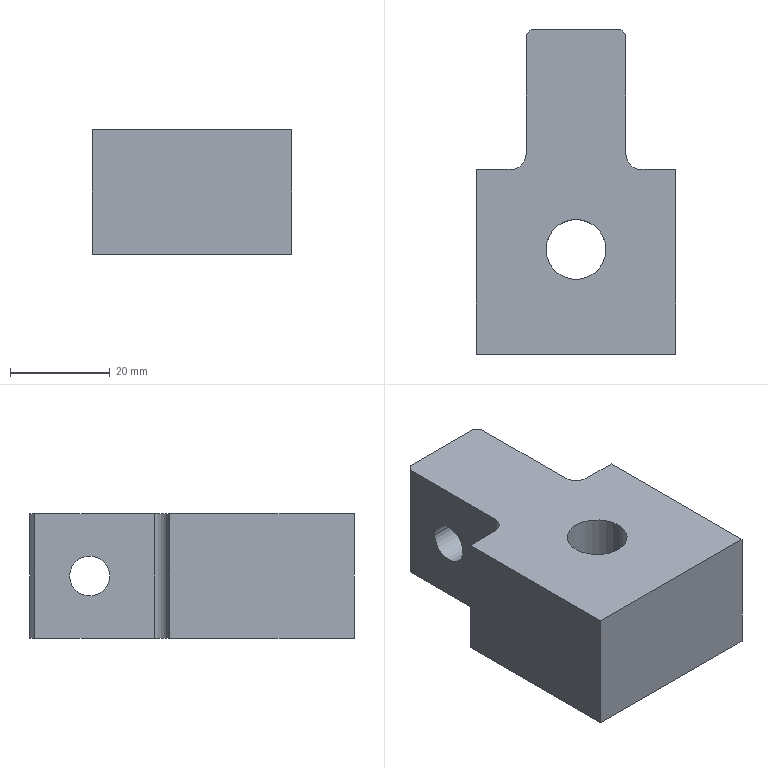Part | STEP file | Chain joint | 1 solid | 18 faces | box 40 x 65 x 25 mm | volume 47239 mm3 | plane 12 | cylinder 6 | commonest cylinder face diameters 6 x2 8 x2 12 x2
STEP:
#1=CARTESIAN_POINT('',(0.,0.,0.));
#2=DIRECTION('',(0.,0.,1.));
#3=DIRECTION('',(1.,0.,0.));
#4=AXIS2_PLACEMENT_3D('',#1,#2,#3);
#5=CARTESIAN_POINT('',(10.,57.,12.5));
#6=VERTEX_POINT('',#5);
#7=CARTESIAN_POINT('',(30.,57.,12.5));
#8=VERTEX_POINT('',#7);
#9=CARTESIAN_POINT('',(0.,57.,12.5));
#10=DIRECTION('',(1.,0.,0.));
#11=VECTOR('',#10,1.);
#12=LINE('',#9,#11);
#13=CARTESIAN_POINT('',(0.,53.,12.5));
#14=DIRECTION('',(1.,0.,0.));
#15=DIRECTION('',(0.,1.,0.));
#16=AXIS2_PLACEMENT_3D('',#13,#14,#15);
#17=CYLINDRICAL_SURFACE('',#16,4.);
#18=CARTESIAN_POINT('',(6.283,0.));
#19=DIRECTION('',(0.,1.));
#20=VECTOR('',#19,1.);
#21=LINE('',#18,#20);
#22=(GEOMETRIC_REPRESENTATION_CONTEXT(2)PARAMETRIC_REPRESENTATION_CONTEXT()REPRESENTATION_CONTEXT('',''));
#23=DEFINITIONAL_REPRESENTATION('',(#21),#22);
#24=PCURVE('',#17,#23);
#25=CARTESIAN_POINT('',(0.,53.,12.5));
#26=DIRECTION('',(1.,0.,0.));
#27=DIRECTION('',(0.,1.,0.));
#28=AXIS2_PLACEMENT_3D('',#25,#26,#27);
#29=CYLINDRICAL_SURFACE('',#28,4.);
#30=CARTESIAN_POINT('',(0.,0.));
#31=DIRECTION('',(0.,1.));
#32=VECTOR('',#31,1.);
#33=LINE('',#30,#32);
#34=(GEOMETRIC_REPRESENTATION_CONTEXT(2)PARAMETRIC_REPRESENTATION_CONTEXT()REPRESENTATION_CONTEXT('',''));
#35=DEFINITIONAL_REPRESENTATION('',(#33),#34);
#36=PCURVE('',#29,#35);
#37=SURFACE_CURVE('',#12,(#24,#36),.PCURVE_S1.);
#38=EDGE_CURVE('',#6,#8,#37,.T.);
#39=ORIENTED_EDGE('',*,*,#38,.T.);
#40=CARTESIAN_POINT('',(30.,49.,12.5));
#41=VERTEX_POINT('',#40);
#42=CARTESIAN_POINT('',(30.,53.,12.5));
#43=DIRECTION('',(1.,0.,0.));
#44=DIRECTION('',(0.,1.,0.));
#45=AXIS2_PLACEMENT_3D('',#42,#43,#44);
#46=CIRCLE('',#45,4.);
#47=CARTESIAN_POINT('',(0.,30.));
#48=DIRECTION('',(1.,0.));
#49=VECTOR('',#48,1.);
#50=LINE('',#47,#49);
#51=(GEOMETRIC_REPRESENTATION_CONTEXT(2)PARAMETRIC_REPRESENTATION_CONTEXT()REPRESENTATION_CONTEXT('',''));
#52=DEFINITIONAL_REPRESENTATION('',(#50),#51);
#53=PCURVE('',#17,#52);
#54=CARTESIAN_POINT('',(30.,65.,25.));
#55=DIRECTION('',(-1.,0.,0.));
#56=DIRECTION('',(0.,-1.,0.));
#57=AXIS2_PLACEMENT_3D('',#54,#55,#56);
#58=PLANE('',#57);
#59=CARTESIAN_POINT('',(8.,-12.5));
#60=CARTESIAN_POINT('',(8.,-5.572));
#61=CARTESIAN_POINT('',(14.,-9.036));
#62=CARTESIAN_POINT('',(20.,-12.5));
#63=CARTESIAN_POINT('',(14.,-15.964));
#64=CARTESIAN_POINT('',(8.,-19.428));
#65=CARTESIAN_POINT('',(8.,-12.5));
#66=(BOUNDED_CURVE()B_SPLINE_CURVE(2,(#59,#60,#61,#62,#63,#64,#65),.UNSPECIFIED.,.T.,.F.)B_SPLINE_CURVE_WITH_KNOTS((1,2,2,2,2,1),(-2.094,0.,2.094,4.189,6.283,8.378),.UNSPECIFIED.)CURVE()GEOMETRIC_REPRESENTATION_ITEM()RATIONAL_B_SPLINE_CURVE((1.,0.5,1.,0.5,1.,0.5,1.))REPRESENTATION_ITEM(''));
#67=(GEOMETRIC_REPRESENTATION_CONTEXT(2)PARAMETRIC_REPRESENTATION_CONTEXT()REPRESENTATION_CONTEXT('',''));
#68=DEFINITIONAL_REPRESENTATION('',(#66),#67);
#69=PCURVE('',#58,#68);
#70=SURFACE_CURVE('',#46,(#53,#69),.PCURVE_S1.);
#71=EDGE_CURVE('',#41,#8,#70,.T.);
#72=ORIENTED_EDGE('',*,*,#71,.F.);
#73=CARTESIAN_POINT('',(10.,49.,12.5));
#74=VERTEX_POINT('',#73);
#75=CARTESIAN_POINT('',(0.,49.,12.5));
#76=DIRECTION('',(1.,0.,0.));
#77=VECTOR('',#76,1.);
#78=LINE('',#75,#77);
#79=CARTESIAN_POINT('',(3.142,0.));
#80=DIRECTION('',(0.,1.));
#81=VECTOR('',#80,1.);
#82=LINE('',#79,#81);
#83=(GEOMETRIC_REPRESENTATION_CONTEXT(2)PARAMETRIC_REPRESENTATION_CONTEXT()REPRESENTATION_CONTEXT('',''));
#84=DEFINITIONAL_REPRESENTATION('',(#82),#83);
#85=PCURVE('',#17,#84);
#86=CARTESIAN_POINT('',(3.142,0.));
#87=DIRECTION('',(0.,1.));
#88=VECTOR('',#87,1.);
#89=LINE('',#86,#88);
#90=(GEOMETRIC_REPRESENTATION_CONTEXT(2)PARAMETRIC_REPRESENTATION_CONTEXT()REPRESENTATION_CONTEXT('',''));
#91=DEFINITIONAL_REPRESENTATION('',(#89),#90);
#92=PCURVE('',#29,#91);
#93=SURFACE_CURVE('',#78,(#85,#92),.PCURVE_S1.);
#94=EDGE_CURVE('',#74,#41,#93,.T.);
#95=ORIENTED_EDGE('',*,*,#94,.F.);
#96=CARTESIAN_POINT('',(10.,53.,12.5));
#97=DIRECTION('',(1.,0.,0.));
#98=DIRECTION('',(0.,0.,-1.));
#99=AXIS2_PLACEMENT_3D('',#96,#97,#98);
#100=CIRCLE('',#99,4.);
#101=CARTESIAN_POINT('',(-1.571,10.));
#102=DIRECTION('',(1.,0.));
#103=VECTOR('',#102,1.);
#104=LINE('',#101,#103);
#105=(GEOMETRIC_REPRESENTATION_CONTEXT(2)PARAMETRIC_REPRESENTATION_CONTEXT()REPRESENTATION_CONTEXT('',''));
#106=DEFINITIONAL_REPRESENTATION('',(#104),#105);
#107=PCURVE('',#17,#106);
#108=CARTESIAN_POINT('',(10.,37.,25.));
#109=DIRECTION('',(1.,0.,0.));
#110=DIRECTION('',(0.,0.,-1.));
#111=AXIS2_PLACEMENT_3D('',#108,#109,#110);
#112=PLANE('',#111);
#113=CARTESIAN_POINT('',(12.5,16.));
#114=DIRECTION('',(1.,0.));
#115=AXIS2_PLACEMENT_2D('',#113,#114);
#116=CIRCLE('',#115,4.);
#117=(GEOMETRIC_REPRESENTATION_CONTEXT(2)PARAMETRIC_REPRESENTATION_CONTEXT()REPRESENTATION_CONTEXT('',''));
#118=DEFINITIONAL_REPRESENTATION('',(#116),#117);
#119=PCURVE('',#112,#118);
#120=SURFACE_CURVE('',#100,(#107,#119),.PCURVE_S1.);
#121=EDGE_CURVE('',#74,#6,#120,.T.);
#122=ORIENTED_EDGE('',*,*,#121,.T.);
#123=EDGE_LOOP('',(#39,#72,#95,#122));
#124=FACE_BOUND('',#123,.F.);
#125=ADVANCED_FACE('',(#124),#17,.F.);
#126=CARTESIAN_POINT('',(14.,21.,25.));
#127=VERTEX_POINT('',#126);
#128=CARTESIAN_POINT('',(14.,21.,0.));
#129=VERTEX_POINT('',#128);
#130=CARTESIAN_POINT('',(14.,21.,25.));
#131=DIRECTION('',(0.,0.,-1.));
#132=VECTOR('',#131,1.);
#133=LINE('',#130,#132);
#134=CARTESIAN_POINT('',(20.,21.,25.));
#135=DIRECTION('',(0.,0.,-1.));
#136=DIRECTION('',(-1.,0.,0.));
#137=AXIS2_PLACEMENT_3D('',#134,#135,#136);
#138=CYLINDRICAL_SURFACE('',#137,6.);
#139=CARTESIAN_POINT('',(6.283,0.));
#140=DIRECTION('',(0.,1.));
#141=VECTOR('',#140,1.);
#142=LINE('',#139,#141);
#143=(GEOMETRIC_REPRESENTATION_CONTEXT(2)PARAMETRIC_REPRESENTATION_CONTEXT()REPRESENTATION_CONTEXT('',''));
#144=DEFINITIONAL_REPRESENTATION('',(#142),#143);
#145=PCURVE('',#138,#144);
#146=CARTESIAN_POINT('',(20.,21.,25.));
#147=DIRECTION('',(0.,0.,-1.));
#148=DIRECTION('',(-1.,0.,0.));
#149=AXIS2_PLACEMENT_3D('',#146,#147,#148);
#150=CYLINDRICAL_SURFACE('',#149,6.);
#151=CARTESIAN_POINT('',(0.,0.));
#152=DIRECTION('',(0.,1.));
#153=VECTOR('',#152,1.);
#154=LINE('',#151,#153);
#155=(GEOMETRIC_REPRESENTATION_CONTEXT(2)PARAMETRIC_REPRESENTATION_CONTEXT()REPRESENTATION_CONTEXT('',''));
#156=DEFINITIONAL_REPRESENTATION('',(#154),#155);
#157=PCURVE('',#150,#156);
#158=SURFACE_CURVE('',#133,(#145,#157),.PCURVE_S1.);
#159=EDGE_CURVE('',#127,#129,#158,.T.);
#160=ORIENTED_EDGE('',*,*,#159,.T.);
#161=CARTESIAN_POINT('',(26.,21.,0.));
#162=VERTEX_POINT('',#161);
#163=CARTESIAN_POINT('',(20.,21.,0.));
#164=DIRECTION('',(0.,0.,1.));
#165=DIRECTION('',(1.,0.,0.));
#166=AXIS2_PLACEMENT_3D('',#163,#164,#165);
#167=CIRCLE('',#166,6.);
#168=CARTESIAN_POINT('',(9.425,25.));
#169=DIRECTION('',(-1.,0.));
#170=VECTOR('',#169,1.);
#171=LINE('',#168,#170);
#172=(GEOMETRIC_REPRESENTATION_CONTEXT(2)PARAMETRIC_REPRESENTATION_CONTEXT()REPRESENTATION_CONTEXT('',''));
#173=DEFINITIONAL_REPRESENTATION('',(#171),#172);
#174=PCURVE('',#138,#173);
#175=CARTESIAN_POINT('',(0.,0.,0.));
#176=DIRECTION('',(0.,0.,-1.));
#177=DIRECTION('',(-1.,0.,0.));
#178=AXIS2_PLACEMENT_3D('',#175,#176,#177);
#179=PLANE('',#178);
#180=CARTESIAN_POINT('',(-26.,21.));
#181=CARTESIAN_POINT('',(-26.,31.392));
#182=CARTESIAN_POINT('',(-17.,26.196));
#183=CARTESIAN_POINT('',(-8.,21.));
#184=CARTESIAN_POINT('',(-17.,15.804));
#185=CARTESIAN_POINT('',(-26.,10.608));
#186=CARTESIAN_POINT('',(-26.,21.));
#187=(BOUNDED_CURVE()B_SPLINE_CURVE(2,(#180,#181,#182,#183,#184,#185,#186),.UNSPECIFIED.,.T.,.F.)B_SPLINE_CURVE_WITH_KNOTS((1,2,2,2,2,1),(-2.094,0.,2.094,4.189,6.283,8.378),.UNSPECIFIED.)CURVE()GEOMETRIC_REPRESENTATION_ITEM()RATIONAL_B_SPLINE_CURVE((1.,0.5,1.,0.5,1.,0.5,1.))REPRESENTATION_ITEM(''));
#188=(GEOMETRIC_REPRESENTATION_CONTEXT(2)PARAMETRIC_REPRESENTATION_CONTEXT()REPRESENTATION_CONTEXT('',''));
#189=DEFINITIONAL_REPRESENTATION('',(#187),#188);
#190=PCURVE('',#179,#189);
#191=SURFACE_CURVE('',#167,(#174,#190),.PCURVE_S1.);
#192=EDGE_CURVE('',#129,#162,#191,.T.);
#193=ORIENTED_EDGE('',*,*,#192,.T.);
#194=CARTESIAN_POINT('',(26.,21.,25.));
#195=VERTEX_POINT('',#194);
#196=CARTESIAN_POINT('',(26.,21.,25.));
#197=DIRECTION('',(0.,0.,-1.));
#198=VECTOR('',#197,1.);
#199=LINE('',#196,#198);
#200=CARTESIAN_POINT('',(3.142,0.));
#201=DIRECTION('',(0.,1.));
#202=VECTOR('',#201,1.);
#203=LINE('',#200,#202);
#204=(GEOMETRIC_REPRESENTATION_CONTEXT(2)PARAMETRIC_REPRESENTATION_CONTEXT()REPRESENTATION_CONTEXT('',''));
#205=DEFINITIONAL_REPRESENTATION('',(#203),#204);
#206=PCURVE('',#138,#205);
#207=CARTESIAN_POINT('',(3.142,0.));
#208=DIRECTION('',(0.,1.));
#209=VECTOR('',#208,1.);
#210=LINE('',#207,#209);
#211=(GEOMETRIC_REPRESENTATION_CONTEXT(2)PARAMETRIC_REPRESENTATION_CONTEXT()REPRESENTATION_CONTEXT('',''));
#212=DEFINITIONAL_REPRESENTATION('',(#210),#211);
#213=PCURVE('',#150,#212);
#214=SURFACE_CURVE('',#199,(#206,#213),.PCURVE_S1.);
#215=EDGE_CURVE('',#195,#162,#214,.T.);
#216=ORIENTED_EDGE('',*,*,#215,.F.);
#217=CARTESIAN_POINT('',(20.,21.,25.));
#218=DIRECTION('',(0.,0.,1.));
#219=DIRECTION('',(1.,0.,0.));
#220=AXIS2_PLACEMENT_3D('',#217,#218,#219);
#221=CIRCLE('',#220,6.);
#222=CARTESIAN_POINT('',(9.425,0.));
#223=DIRECTION('',(-1.,0.));
#224=VECTOR('',#223,1.);
#225=LINE('',#222,#224);
#226=(GEOMETRIC_REPRESENTATION_CONTEXT(2)PARAMETRIC_REPRESENTATION_CONTEXT()REPRESENTATION_CONTEXT('',''));
#227=DEFINITIONAL_REPRESENTATION('',(#225),#226);
#228=PCURVE('',#138,#227);
#229=CARTESIAN_POINT('',(0.,0.,25.));
#230=DIRECTION('',(0.,0.,-1.));
#231=DIRECTION('',(-1.,0.,0.));
#232=AXIS2_PLACEMENT_3D('',#229,#230,#231);
#233=PLANE('',#232);
#234=CARTESIAN_POINT('',(-26.,21.));
#235=CARTESIAN_POINT('',(-26.,31.392));
#236=CARTESIAN_POINT('',(-17.,26.196));
#237=CARTESIAN_POINT('',(-8.,21.));
#238=CARTESIAN_POINT('',(-17.,15.804));
#239=CARTESIAN_POINT('',(-26.,10.608));
#240=CARTESIAN_POINT('',(-26.,21.));
#241=(BOUNDED_CURVE()B_SPLINE_CURVE(2,(#234,#235,#236,#237,#238,#239,#240),.UNSPECIFIED.,.T.,.F.)B_SPLINE_CURVE_WITH_KNOTS((1,2,2,2,2,1),(-2.094,0.,2.094,4.189,6.283,8.378),.UNSPECIFIED.)CURVE()GEOMETRIC_REPRESENTATION_ITEM()RATIONAL_B_SPLINE_CURVE((1.,0.5,1.,0.5,1.,0.5,1.))REPRESENTATION_ITEM(''));
#242=(GEOMETRIC_REPRESENTATION_CONTEXT(2)PARAMETRIC_REPRESENTATION_CONTEXT()REPRESENTATION_CONTEXT('',''));
#243=DEFINITIONAL_REPRESENTATION('',(#241),#242);
#244=PCURVE('',#233,#243);
#245=SURFACE_CURVE('',#221,(#228,#244),.PCURVE_S1.);
#246=EDGE_CURVE('',#127,#195,#245,.T.);
#247=ORIENTED_EDGE('',*,*,#246,.F.);
#248=EDGE_LOOP('',(#160,#193,#216,#247));
#249=FACE_BOUND('',#248,.F.);
#250=ADVANCED_FACE('',(#249),#138,.F.);
#251=CARTESIAN_POINT('',(29.,65.,25.));
#252=VERTEX_POINT('',#251);
#253=CARTESIAN_POINT('',(11.,65.,25.));
#254=VERTEX_POINT('',#253);
#255=CARTESIAN_POINT('',(10.,65.,25.));
#256=DIRECTION('',(-1.,0.,0.));
#257=VECTOR('',#256,1.);
#258=LINE('',#255,#257);
#259=CARTESIAN_POINT('',(-10.,65.));
#260=DIRECTION('',(1.,0.));
#261=VECTOR('',#260,1.);
#262=LINE('',#259,#261);
#263=(GEOMETRIC_REPRESENTATION_CONTEXT(2)PARAMETRIC_REPRESENTATION_CONTEXT()REPRESENTATION_CONTEXT('',''));
#264=DEFINITIONAL_REPRESENTATION('',(#262),#263);
#265=PCURVE('',#233,#264);
#266=CARTESIAN_POINT('',(10.,65.,25.));
#267=DIRECTION('',(0.,-1.,0.));
#268=DIRECTION('',(0.,0.,-1.));
#269=AXIS2_PLACEMENT_3D('',#266,#267,#268);
#270=PLANE('',#269);
#271=CARTESIAN_POINT('',(0.,0.));
#272=DIRECTION('',(0.,-1.));
#273=VECTOR('',#272,1.);
#274=LINE('',#271,#273);
#275=(GEOMETRIC_REPRESENTATION_CONTEXT(2)PARAMETRIC_REPRESENTATION_CONTEXT()REPRESENTATION_CONTEXT('',''));
#276=DEFINITIONAL_REPRESENTATION('',(#274),#275);
#277=PCURVE('',#270,#276);
#278=SURFACE_CURVE('',#258,(#265,#277),.PCURVE_S1.);
#279=EDGE_CURVE('',#252,#254,#278,.T.);
#280=ORIENTED_EDGE('',*,*,#279,.T.);
#281=CARTESIAN_POINT('',(10.,64.,25.));
#282=VERTEX_POINT('',#281);
#283=CARTESIAN_POINT('',(10.,64.,25.));
#284=DIRECTION('',(-0.7071,-0.7071,0.));
#285=VECTOR('',#284,1.);
#286=LINE('',#283,#285);
#287=CARTESIAN_POINT('',(-10.,64.));
#288=DIRECTION('',(0.7071,-0.7071));
#289=VECTOR('',#288,1.);
#290=LINE('',#287,#289);
#291=(GEOMETRIC_REPRESENTATION_CONTEXT(2)PARAMETRIC_REPRESENTATION_CONTEXT()REPRESENTATION_CONTEXT('',''));
#292=DEFINITIONAL_REPRESENTATION('',(#290),#291);
#293=PCURVE('',#233,#292);
#294=CARTESIAN_POINT('',(10.,64.,25.));
#295=DIRECTION('',(0.7071,-0.7071,0.));
#296=DIRECTION('',(0.,0.,-1.));
#297=AXIS2_PLACEMENT_3D('',#294,#295,#296);
#298=PLANE('',#297);
#299=CARTESIAN_POINT('',(0.,0.));
#300=DIRECTION('',(0.,-1.));
#301=VECTOR('',#300,1.);
#302=LINE('',#299,#301);
#303=(GEOMETRIC_REPRESENTATION_CONTEXT(2)PARAMETRIC_REPRESENTATION_CONTEXT()REPRESENTATION_CONTEXT('',''));
#304=DEFINITIONAL_REPRESENTATION('',(#302),#303);
#305=PCURVE('',#298,#304);
#306=SURFACE_CURVE('',#286,(#293,#305),.PCURVE_S1.);
#307=EDGE_CURVE('',#254,#282,#306,.T.);
#308=ORIENTED_EDGE('',*,*,#307,.T.);
#309=CARTESIAN_POINT('',(10.,40.,25.));
#310=VERTEX_POINT('',#309);
#311=CARTESIAN_POINT('',(10.,37.,25.));
#312=DIRECTION('',(0.,-1.,0.));
#313=VECTOR('',#312,1.);
#314=LINE('',#311,#313);
#315=CARTESIAN_POINT('',(-10.,37.));
#316=DIRECTION('',(0.,-1.));
#317=VECTOR('',#316,1.);
#318=LINE('',#315,#317);
#319=(GEOMETRIC_REPRESENTATION_CONTEXT(2)PARAMETRIC_REPRESENTATION_CONTEXT()REPRESENTATION_CONTEXT('',''));
#320=DEFINITIONAL_REPRESENTATION('',(#318),#319);
#321=PCURVE('',#233,#320);
#322=CARTESIAN_POINT('',(0.,0.));
#323=DIRECTION('',(0.,-1.));
#324=VECTOR('',#323,1.);
#325=LINE('',#322,#324);
#326=(GEOMETRIC_REPRESENTATION_CONTEXT(2)PARAMETRIC_REPRESENTATION_CONTEXT()REPRESENTATION_CONTEXT('',''));
#327=DEFINITIONAL_REPRESENTATION('',(#325),#326);
#328=PCURVE('',#112,#327);
#329=SURFACE_CURVE('',#314,(#321,#328),.PCURVE_S1.);
#330=EDGE_CURVE('',#282,#310,#329,.T.);
#331=ORIENTED_EDGE('',*,*,#330,.T.);
#332=CARTESIAN_POINT('',(7.,37.,25.));
#333=VERTEX_POINT('',#332);
#334=CARTESIAN_POINT('',(7.,40.,25.));
#335=DIRECTION('',(0.,0.,-1.));
#336=DIRECTION('',(-1.,0.,0.));
#337=AXIS2_PLACEMENT_3D('',#334,#335,#336);
#338=CIRCLE('',#337,3.);
#339=CARTESIAN_POINT('',(-7.,40.));
#340=DIRECTION('',(1.,0.));
#341=AXIS2_PLACEMENT_2D('',#339,#340);
#342=CIRCLE('',#341,3.);
#343=(GEOMETRIC_REPRESENTATION_CONTEXT(2)PARAMETRIC_REPRESENTATION_CONTEXT()REPRESENTATION_CONTEXT('',''));
#344=DEFINITIONAL_REPRESENTATION('',(#342),#343);
#345=PCURVE('',#233,#344);
#346=CARTESIAN_POINT('',(7.,40.,25.));
#347=DIRECTION('',(0.,0.,1.));
#348=DIRECTION('',(1.,0.,0.));
#349=AXIS2_PLACEMENT_3D('',#346,#347,#348);
#350=CYLINDRICAL_SURFACE('',#349,3.);
#351=CARTESIAN_POINT('',(9.425,0.));
#352=DIRECTION('',(-1.,0.));
#353=VECTOR('',#352,1.);
#354=LINE('',#351,#353);
#355=(GEOMETRIC_REPRESENTATION_CONTEXT(2)PARAMETRIC_REPRESENTATION_CONTEXT()REPRESENTATION_CONTEXT('',''));
#356=DEFINITIONAL_REPRESENTATION('',(#354),#355);
#357=PCURVE('',#350,#356);
#358=SURFACE_CURVE('',#338,(#345,#357),.PCURVE_S1.);
#359=EDGE_CURVE('',#310,#333,#358,.T.);
#360=ORIENTED_EDGE('',*,*,#359,.T.);
#361=CARTESIAN_POINT('',(0.,37.,25.));
#362=VERTEX_POINT('',#361);
#363=CARTESIAN_POINT('',(0.,37.,25.));
#364=DIRECTION('',(-1.,0.,0.));
#365=VECTOR('',#364,1.);
#366=LINE('',#363,#365);
#367=CARTESIAN_POINT('',(0.,37.));
#368=DIRECTION('',(1.,0.));
#369=VECTOR('',#368,1.);
#370=LINE('',#367,#369);
#371=(GEOMETRIC_REPRESENTATION_CONTEXT(2)PARAMETRIC_REPRESENTATION_CONTEXT()REPRESENTATION_CONTEXT('',''));
#372=DEFINITIONAL_REPRESENTATION('',(#370),#371);
#373=PCURVE('',#233,#372);
#374=CARTESIAN_POINT('',(0.,37.,25.));
#375=DIRECTION('',(0.,-1.,0.));
#376=DIRECTION('',(0.,0.,-1.));
#377=AXIS2_PLACEMENT_3D('',#374,#375,#376);
#378=PLANE('',#377);
#379=CARTESIAN_POINT('',(0.,0.));
#380=DIRECTION('',(0.,-1.));
#381=VECTOR('',#380,1.);
#382=LINE('',#379,#381);
#383=(GEOMETRIC_REPRESENTATION_CONTEXT(2)PARAMETRIC_REPRESENTATION_CONTEXT()REPRESENTATION_CONTEXT('',''));
#384=DEFINITIONAL_REPRESENTATION('',(#382),#383);
#385=PCURVE('',#378,#384);
#386=SURFACE_CURVE('',#366,(#373,#385),.PCURVE_S1.);
#387=EDGE_CURVE('',#333,#362,#386,.T.);
#388=ORIENTED_EDGE('',*,*,#387,.T.);
#389=CARTESIAN_POINT('',(0.,0.,25.));
#390=VERTEX_POINT('',#389);
#391=CARTESIAN_POINT('',(0.,0.,25.));
#392=DIRECTION('',(0.,-1.,0.));
#393=VECTOR('',#392,1.);
#394=LINE('',#391,#393);
#395=CARTESIAN_POINT('',(0.,0.));
#396=DIRECTION('',(0.,-1.));
#397=VECTOR('',#396,1.);
#398=LINE('',#395,#397);
#399=(GEOMETRIC_REPRESENTATION_CONTEXT(2)PARAMETRIC_REPRESENTATION_CONTEXT()REPRESENTATION_CONTEXT('',''));
#400=DEFINITIONAL_REPRESENTATION('',(#398),#399);
#401=PCURVE('',#233,#400);
#402=CARTESIAN_POINT('',(0.,0.,25.));
#403=DIRECTION('',(1.,0.,0.));
#404=DIRECTION('',(0.,0.,-1.));
#405=AXIS2_PLACEMENT_3D('',#402,#403,#404);
#406=PLANE('',#405);
#407=CARTESIAN_POINT('',(0.,0.));
#408=DIRECTION('',(0.,-1.));
#409=VECTOR('',#408,1.);
#410=LINE('',#407,#409);
#411=(GEOMETRIC_REPRESENTATION_CONTEXT(2)PARAMETRIC_REPRESENTATION_CONTEXT()REPRESENTATION_CONTEXT('',''));
#412=DEFINITIONAL_REPRESENTATION('',(#410),#411);
#413=PCURVE('',#406,#412);
#414=SURFACE_CURVE('',#394,(#401,#413),.PCURVE_S1.);
#415=EDGE_CURVE('',#362,#390,#414,.T.);
#416=ORIENTED_EDGE('',*,*,#415,.T.);
#417=CARTESIAN_POINT('',(40.,0.,25.));
#418=VERTEX_POINT('',#417);
#419=CARTESIAN_POINT('',(0.,0.,25.));
#420=DIRECTION('',(1.,0.,0.));
#421=VECTOR('',#420,1.);
#422=LINE('',#419,#421);
#423=CARTESIAN_POINT('',(0.,0.));
#424=DIRECTION('',(-1.,0.));
#425=VECTOR('',#424,1.);
#426=LINE('',#423,#425);
#427=(GEOMETRIC_REPRESENTATION_CONTEXT(2)PARAMETRIC_REPRESENTATION_CONTEXT()REPRESENTATION_CONTEXT('',''));
#428=DEFINITIONAL_REPRESENTATION('',(#426),#427);
#429=PCURVE('',#233,#428);
#430=CARTESIAN_POINT('',(0.,0.,25.));
#431=DIRECTION('',(0.,1.,0.));
#432=DIRECTION('',(0.,0.,1.));
#433=AXIS2_PLACEMENT_3D('',#430,#431,#432);
#434=PLANE('',#433);
#435=CARTESIAN_POINT('',(0.,0.));
#436=DIRECTION('',(0.,1.));
#437=VECTOR('',#436,1.);
#438=LINE('',#435,#437);
#439=(GEOMETRIC_REPRESENTATION_CONTEXT(2)PARAMETRIC_REPRESENTATION_CONTEXT()REPRESENTATION_CONTEXT('',''));
#440=DEFINITIONAL_REPRESENTATION('',(#438),#439);
#441=PCURVE('',#434,#440);
#442=SURFACE_CURVE('',#422,(#429,#441),.PCURVE_S1.);
#443=EDGE_CURVE('',#390,#418,#442,.T.);
#444=ORIENTED_EDGE('',*,*,#443,.T.);
#445=CARTESIAN_POINT('',(40.,37.,25.));
#446=VERTEX_POINT('',#445);
#447=CARTESIAN_POINT('',(40.,0.,25.));
#448=DIRECTION('',(0.,1.,0.));
#449=VECTOR('',#448,1.);
#450=LINE('',#447,#449);
#451=CARTESIAN_POINT('',(-40.,0.));
#452=DIRECTION('',(0.,1.));
#453=VECTOR('',#452,1.);
#454=LINE('',#451,#453);
#455=(GEOMETRIC_REPRESENTATION_CONTEXT(2)PARAMETRIC_REPRESENTATION_CONTEXT()REPRESENTATION_CONTEXT('',''));
#456=DEFINITIONAL_REPRESENTATION('',(#454),#455);
#457=PCURVE('',#233,#456);
#458=CARTESIAN_POINT('',(40.,0.,25.));
#459=DIRECTION('',(-1.,0.,0.));
#460=DIRECTION('',(0.,0.,1.));
#461=AXIS2_PLACEMENT_3D('',#458,#459,#460);
#462=PLANE('',#461);
#463=CARTESIAN_POINT('',(0.,0.));
#464=DIRECTION('',(0.,1.));
#465=VECTOR('',#464,1.);
#466=LINE('',#463,#465);
#467=(GEOMETRIC_REPRESENTATION_CONTEXT(2)PARAMETRIC_REPRESENTATION_CONTEXT()REPRESENTATION_CONTEXT('',''));
#468=DEFINITIONAL_REPRESENTATION('',(#466),#467);
#469=PCURVE('',#462,#468);
#470=SURFACE_CURVE('',#450,(#457,#469),.PCURVE_S1.);
#471=EDGE_CURVE('',#418,#446,#470,.T.);
#472=ORIENTED_EDGE('',*,*,#471,.T.);
#473=CARTESIAN_POINT('',(33.,37.,25.));
#474=VERTEX_POINT('',#473);
#475=CARTESIAN_POINT('',(30.,37.,25.));
#476=DIRECTION('',(-1.,0.,0.));
#477=VECTOR('',#476,1.);
#478=LINE('',#475,#477);
#479=CARTESIAN_POINT('',(-30.,37.));
#480=DIRECTION('',(1.,0.));
#481=VECTOR('',#480,1.);
#482=LINE('',#479,#481);
#483=(GEOMETRIC_REPRESENTATION_CONTEXT(2)PARAMETRIC_REPRESENTATION_CONTEXT()REPRESENTATION_CONTEXT('',''));
#484=DEFINITIONAL_REPRESENTATION('',(#482),#483);
#485=PCURVE('',#233,#484);
#486=CARTESIAN_POINT('',(30.,37.,25.));
#487=DIRECTION('',(0.,-1.,0.));
#488=DIRECTION('',(0.,0.,-1.));
#489=AXIS2_PLACEMENT_3D('',#486,#487,#488);
#490=PLANE('',#489);
#491=CARTESIAN_POINT('',(0.,0.));
#492=DIRECTION('',(0.,-1.));
#493=VECTOR('',#492,1.);
#494=LINE('',#491,#493);
#495=(GEOMETRIC_REPRESENTATION_CONTEXT(2)PARAMETRIC_REPRESENTATION_CONTEXT()REPRESENTATION_CONTEXT('',''));
#496=DEFINITIONAL_REPRESENTATION('',(#494),#495);
#497=PCURVE('',#490,#496);
#498=SURFACE_CURVE('',#478,(#485,#497),.PCURVE_S1.);
#499=EDGE_CURVE('',#446,#474,#498,.T.);
#500=ORIENTED_EDGE('',*,*,#499,.T.);
#501=CARTESIAN_POINT('',(30.,40.,25.));
#502=VERTEX_POINT('',#501);
#503=CARTESIAN_POINT('',(33.,40.,25.));
#504=DIRECTION('',(0.,0.,-1.));
#505=DIRECTION('',(-1.,0.,0.));
#506=AXIS2_PLACEMENT_3D('',#503,#504,#505);
#507=CIRCLE('',#506,3.);
#508=CARTESIAN_POINT('',(-33.,40.));
#509=DIRECTION('',(1.,0.));
#510=AXIS2_PLACEMENT_2D('',#508,#509);
#511=CIRCLE('',#510,3.);
#512=(GEOMETRIC_REPRESENTATION_CONTEXT(2)PARAMETRIC_REPRESENTATION_CONTEXT()REPRESENTATION_CONTEXT('',''));
#513=DEFINITIONAL_REPRESENTATION('',(#511),#512);
#514=PCURVE('',#233,#513);
#515=CARTESIAN_POINT('',(33.,40.,25.));
#516=DIRECTION('',(0.,0.,1.));
#517=DIRECTION('',(1.,0.,0.));
#518=AXIS2_PLACEMENT_3D('',#515,#516,#517);
#519=CYLINDRICAL_SURFACE('',#518,3.);
#520=CARTESIAN_POINT('',(9.425,0.));
#521=DIRECTION('',(-1.,0.));
#522=VECTOR('',#521,1.);
#523=LINE('',#520,#522);
#524=(GEOMETRIC_REPRESENTATION_CONTEXT(2)PARAMETRIC_REPRESENTATION_CONTEXT()REPRESENTATION_CONTEXT('',''));
#525=DEFINITIONAL_REPRESENTATION('',(#523),#524);
#526=PCURVE('',#519,#525);
#527=SURFACE_CURVE('',#507,(#514,#526),.PCURVE_S1.);
#528=EDGE_CURVE('',#474,#502,#527,.T.);
#529=ORIENTED_EDGE('',*,*,#528,.T.);
#530=CARTESIAN_POINT('',(30.,64.,25.));
#531=VERTEX_POINT('',#530);
#532=CARTESIAN_POINT('',(30.,65.,25.));
#533=DIRECTION('',(0.,1.,0.));
#534=VECTOR('',#533,1.);
#535=LINE('',#532,#534);
#536=CARTESIAN_POINT('',(-30.,65.));
#537=DIRECTION('',(0.,1.));
#538=VECTOR('',#537,1.);
#539=LINE('',#536,#538);
#540=(GEOMETRIC_REPRESENTATION_CONTEXT(2)PARAMETRIC_REPRESENTATION_CONTEXT()REPRESENTATION_CONTEXT('',''));
#541=DEFINITIONAL_REPRESENTATION('',(#539),#540);
#542=PCURVE('',#233,#541);
#543=CARTESIAN_POINT('',(0.,0.));
#544=DIRECTION('',(-1.,0.));
#545=VECTOR('',#544,1.);
#546=LINE('',#543,#545);
#547=(GEOMETRIC_REPRESENTATION_CONTEXT(2)PARAMETRIC_REPRESENTATION_CONTEXT()REPRESENTATION_CONTEXT('',''));
#548=DEFINITIONAL_REPRESENTATION('',(#546),#547);
#549=PCURVE('',#58,#548);
#550=SURFACE_CURVE('',#535,(#542,#549),.PCURVE_S1.);
#551=EDGE_CURVE('',#502,#531,#550,.T.);
#552=ORIENTED_EDGE('',*,*,#551,.T.);
#553=CARTESIAN_POINT('',(29.,65.,25.));
#554=DIRECTION('',(-0.7071,0.7071,0.));
#555=VECTOR('',#554,1.);
#556=LINE('',#553,#555);
#557=CARTESIAN_POINT('',(-29.,65.));
#558=DIRECTION('',(0.7071,0.7071));
#559=VECTOR('',#558,1.);
#560=LINE('',#557,#559);
#561=(GEOMETRIC_REPRESENTATION_CONTEXT(2)PARAMETRIC_REPRESENTATION_CONTEXT()REPRESENTATION_CONTEXT('',''));
#562=DEFINITIONAL_REPRESENTATION('',(#560),#561);
#563=PCURVE('',#233,#562);
#564=CARTESIAN_POINT('',(29.,65.,25.));
#565=DIRECTION('',(-0.7071,-0.7071,0.));
#566=DIRECTION('',(0.,0.,-1.));
#567=AXIS2_PLACEMENT_3D('',#564,#565,#566);
#568=PLANE('',#567);
#569=CARTESIAN_POINT('',(0.,0.));
#570=DIRECTION('',(0.,-1.));
#571=VECTOR('',#570,1.);
#572=LINE('',#569,#571);
#573=(GEOMETRIC_REPRESENTATION_CONTEXT(2)PARAMETRIC_REPRESENTATION_CONTEXT()REPRESENTATION_CONTEXT('',''));
#574=DEFINITIONAL_REPRESENTATION('',(#572),#573);
#575=PCURVE('',#568,#574);
#576=SURFACE_CURVE('',#556,(#563,#575),.PCURVE_S1.);
#577=EDGE_CURVE('',#531,#252,#576,.T.);
#578=ORIENTED_EDGE('',*,*,#577,.T.);
#579=EDGE_LOOP('',(#280,#308,#331,#360,#388,#416,#444,#472,#500,#529,#552,#578));
#580=FACE_BOUND('',#579,.T.);
#581=ORIENTED_EDGE('',*,*,#246,.F.);
#582=CARTESIAN_POINT('',(20.,21.,25.));
#583=DIRECTION('',(0.,0.,1.));
#584=DIRECTION('',(1.,0.,0.));
#585=AXIS2_PLACEMENT_3D('',#582,#583,#584);
#586=CIRCLE('',#585,6.);
#587=CARTESIAN_POINT('',(-26.,21.));
#588=CARTESIAN_POINT('',(-26.,31.392));
#589=CARTESIAN_POINT('',(-17.,26.196));
#590=CARTESIAN_POINT('',(-8.,21.));
#591=CARTESIAN_POINT('',(-17.,15.804));
#592=CARTESIAN_POINT('',(-26.,10.608));
#593=CARTESIAN_POINT('',(-26.,21.));
#594=(BOUNDED_CURVE()B_SPLINE_CURVE(2,(#587,#588,#589,#590,#591,#592,#593),.UNSPECIFIED.,.T.,.F.)B_SPLINE_CURVE_WITH_KNOTS((1,2,2,2,2,1),(-2.094,0.,2.094,4.189,6.283,8.378),.UNSPECIFIED.)CURVE()GEOMETRIC_REPRESENTATION_ITEM()RATIONAL_B_SPLINE_CURVE((1.,0.5,1.,0.5,1.,0.5,1.))REPRESENTATION_ITEM(''));
#595=(GEOMETRIC_REPRESENTATION_CONTEXT(2)PARAMETRIC_REPRESENTATION_CONTEXT()REPRESENTATION_CONTEXT('',''));
#596=DEFINITIONAL_REPRESENTATION('',(#594),#595);
#597=PCURVE('',#233,#596);
#598=CARTESIAN_POINT('',(3.142,0.));
#599=DIRECTION('',(-1.,0.));
#600=VECTOR('',#599,1.);
#601=LINE('',#598,#600);
#602=(GEOMETRIC_REPRESENTATION_CONTEXT(2)PARAMETRIC_REPRESENTATION_CONTEXT()REPRESENTATION_CONTEXT('',''));
#603=DEFINITIONAL_REPRESENTATION('',(#601),#602);
#604=PCURVE('',#150,#603);
#605=SURFACE_CURVE('',#586,(#597,#604),.PCURVE_S1.);
#606=EDGE_CURVE('',#195,#127,#605,.T.);
#607=ORIENTED_EDGE('',*,*,#606,.F.);
#608=EDGE_LOOP('',(#581,#607));
#609=FACE_BOUND('',#608,.T.);
#610=ADVANCED_FACE('',(#580,#609),#233,.F.);
#611=CARTESIAN_POINT('',(10.,64.,0.));
#612=VERTEX_POINT('',#611);
#613=CARTESIAN_POINT('',(10.,40.,0.));
#614=VERTEX_POINT('',#613);
#615=CARTESIAN_POINT('',(10.,37.,0.));
#616=DIRECTION('',(0.,-1.,0.));
#617=VECTOR('',#616,1.);
#618=LINE('',#615,#617);
#619=CARTESIAN_POINT('',(-10.,37.));
#620=DIRECTION('',(0.,-1.));
#621=VECTOR('',#620,1.);
#622=LINE('',#619,#621);
#623=(GEOMETRIC_REPRESENTATION_CONTEXT(2)PARAMETRIC_REPRESENTATION_CONTEXT()REPRESENTATION_CONTEXT('',''));
#624=DEFINITIONAL_REPRESENTATION('',(#622),#623);
#625=PCURVE('',#179,#624);
#626=CARTESIAN_POINT('',(25.,0.));
#627=DIRECTION('',(0.,-1.));
#628=VECTOR('',#627,1.);
#629=LINE('',#626,#628);
#630=(GEOMETRIC_REPRESENTATION_CONTEXT(2)PARAMETRIC_REPRESENTATION_CONTEXT()REPRESENTATION_CONTEXT('',''));
#631=DEFINITIONAL_REPRESENTATION('',(#629),#630);
#632=PCURVE('',#112,#631);
#633=SURFACE_CURVE('',#618,(#625,#632),.PCURVE_S1.);
#634=EDGE_CURVE('',#612,#614,#633,.T.);
#635=ORIENTED_EDGE('',*,*,#634,.F.);
#636=CARTESIAN_POINT('',(11.,65.,0.));
#637=VERTEX_POINT('',#636);
#638=CARTESIAN_POINT('',(-27.,27.,0.));
#639=DIRECTION('',(0.7071,0.7071,0.));
#640=VECTOR('',#639,1.);
#641=LINE('',#638,#640);
#642=CARTESIAN_POINT('',(27.,27.));
#643=DIRECTION('',(-0.7071,0.7071));
#644=VECTOR('',#643,1.);
#645=LINE('',#642,#644);
#646=(GEOMETRIC_REPRESENTATION_CONTEXT(2)PARAMETRIC_REPRESENTATION_CONTEXT()REPRESENTATION_CONTEXT('',''));
#647=DEFINITIONAL_REPRESENTATION('',(#645),#646);
#648=PCURVE('',#179,#647);
#649=CARTESIAN_POINT('',(25.,-52.326));
#650=DIRECTION('',(0.,1.));
#651=VECTOR('',#650,1.);
#652=LINE('',#649,#651);
#653=(GEOMETRIC_REPRESENTATION_CONTEXT(2)PARAMETRIC_REPRESENTATION_CONTEXT()REPRESENTATION_CONTEXT('',''));
#654=DEFINITIONAL_REPRESENTATION('',(#652),#653);
#655=PCURVE('',#298,#654);
#656=SURFACE_CURVE('',#641,(#648,#655),.PCURVE_S1.);
#657=EDGE_CURVE('',#612,#637,#656,.T.);
#658=ORIENTED_EDGE('',*,*,#657,.T.);
#659=CARTESIAN_POINT('',(29.,65.,0.));
#660=VERTEX_POINT('',#659);
#661=CARTESIAN_POINT('',(10.,65.,0.));
#662=DIRECTION('',(-1.,0.,0.));
#663=VECTOR('',#662,1.);
#664=LINE('',#661,#663);
#665=CARTESIAN_POINT('',(-10.,65.));
#666=DIRECTION('',(1.,0.));
#667=VECTOR('',#666,1.);
#668=LINE('',#665,#667);
#669=(GEOMETRIC_REPRESENTATION_CONTEXT(2)PARAMETRIC_REPRESENTATION_CONTEXT()REPRESENTATION_CONTEXT('',''));
#670=DEFINITIONAL_REPRESENTATION('',(#668),#669);
#671=PCURVE('',#179,#670);
#672=CARTESIAN_POINT('',(25.,0.));
#673=DIRECTION('',(0.,-1.));
#674=VECTOR('',#673,1.);
#675=LINE('',#672,#674);
#676=(GEOMETRIC_REPRESENTATION_CONTEXT(2)PARAMETRIC_REPRESENTATION_CONTEXT()REPRESENTATION_CONTEXT('',''));
#677=DEFINITIONAL_REPRESENTATION('',(#675),#676);
#678=PCURVE('',#270,#677);
#679=SURFACE_CURVE('',#664,(#671,#678),.PCURVE_S1.);
#680=EDGE_CURVE('',#660,#637,#679,.T.);
#681=ORIENTED_EDGE('',*,*,#680,.F.);
#682=CARTESIAN_POINT('',(30.,64.,0.));
#683=VERTEX_POINT('',#682);
#684=CARTESIAN_POINT('',(47.,47.,0.));
#685=DIRECTION('',(0.7071,-0.7071,0.));
#686=VECTOR('',#685,1.);
#687=LINE('',#684,#686);
#688=CARTESIAN_POINT('',(-47.,47.));
#689=DIRECTION('',(-0.7071,-0.7071));
#690=VECTOR('',#689,1.);
#691=LINE('',#688,#690);
#692=(GEOMETRIC_REPRESENTATION_CONTEXT(2)PARAMETRIC_REPRESENTATION_CONTEXT()REPRESENTATION_CONTEXT('',''));
#693=DEFINITIONAL_REPRESENTATION('',(#691),#692);
#694=PCURVE('',#179,#693);
#695=CARTESIAN_POINT('',(25.,25.456));
#696=DIRECTION('',(0.,1.));
#697=VECTOR('',#696,1.);
#698=LINE('',#695,#697);
#699=(GEOMETRIC_REPRESENTATION_CONTEXT(2)PARAMETRIC_REPRESENTATION_CONTEXT()REPRESENTATION_CONTEXT('',''));
#700=DEFINITIONAL_REPRESENTATION('',(#698),#699);
#701=PCURVE('',#568,#700);
#702=SURFACE_CURVE('',#687,(#694,#701),.PCURVE_S1.);
#703=EDGE_CURVE('',#660,#683,#702,.T.);
#704=ORIENTED_EDGE('',*,*,#703,.T.);
#705=CARTESIAN_POINT('',(30.,40.,0.));
#706=VERTEX_POINT('',#705);
#707=CARTESIAN_POINT('',(30.,65.,0.));
#708=DIRECTION('',(0.,1.,0.));
#709=VECTOR('',#708,1.);
#710=LINE('',#707,#709);
#711=CARTESIAN_POINT('',(-30.,65.));
#712=DIRECTION('',(0.,1.));
#713=VECTOR('',#712,1.);
#714=LINE('',#711,#713);
#715=(GEOMETRIC_REPRESENTATION_CONTEXT(2)PARAMETRIC_REPRESENTATION_CONTEXT()REPRESENTATION_CONTEXT('',''));
#716=DEFINITIONAL_REPRESENTATION('',(#714),#715);
#717=PCURVE('',#179,#716);
#718=CARTESIAN_POINT('',(0.,-25.));
#719=DIRECTION('',(-1.,0.));
#720=VECTOR('',#719,1.);
#721=LINE('',#718,#720);
#722=(GEOMETRIC_REPRESENTATION_CONTEXT(2)PARAMETRIC_REPRESENTATION_CONTEXT()REPRESENTATION_CONTEXT('',''));
#723=DEFINITIONAL_REPRESENTATION('',(#721),#722);
#724=PCURVE('',#58,#723);
#725=SURFACE_CURVE('',#710,(#717,#724),.PCURVE_S1.);
#726=EDGE_CURVE('',#706,#683,#725,.T.);
#727=ORIENTED_EDGE('',*,*,#726,.F.);
#728=CARTESIAN_POINT('',(33.,37.,0.));
#729=VERTEX_POINT('',#728);
#730=CARTESIAN_POINT('',(33.,40.,0.));
#731=DIRECTION('',(0.,0.,1.));
#732=DIRECTION('',(-1.,0.,0.));
#733=AXIS2_PLACEMENT_3D('',#730,#731,#732);
#734=CIRCLE('',#733,3.);
#735=CARTESIAN_POINT('',(-30.,40.));
#736=CARTESIAN_POINT('',(-30.,34.804));
#737=CARTESIAN_POINT('',(-34.5,37.402));
#738=CARTESIAN_POINT('',(-39.,40.));
#739=CARTESIAN_POINT('',(-34.5,42.598));
#740=CARTESIAN_POINT('',(-30.,45.196));
#741=CARTESIAN_POINT('',(-30.,40.));
#742=(BOUNDED_CURVE()B_SPLINE_CURVE(2,(#735,#736,#737,#738,#739,#740,#741),.UNSPECIFIED.,.T.,.F.)B_SPLINE_CURVE_WITH_KNOTS((1,2,2,2,2,1),(-2.094,0.,2.094,4.189,6.283,8.378),.UNSPECIFIED.)CURVE()GEOMETRIC_REPRESENTATION_ITEM()RATIONAL_B_SPLINE_CURVE((1.,0.5,1.,0.5,1.,0.5,1.))REPRESENTATION_ITEM(''));
#743=(GEOMETRIC_REPRESENTATION_CONTEXT(2)PARAMETRIC_REPRESENTATION_CONTEXT()REPRESENTATION_CONTEXT('',''));
#744=DEFINITIONAL_REPRESENTATION('',(#742),#743);
#745=PCURVE('',#179,#744);
#746=CARTESIAN_POINT('',(3.142,-25.));
#747=DIRECTION('',(1.,0.));
#748=VECTOR('',#747,1.);
#749=LINE('',#746,#748);
#750=(GEOMETRIC_REPRESENTATION_CONTEXT(2)PARAMETRIC_REPRESENTATION_CONTEXT()REPRESENTATION_CONTEXT('',''));
#751=DEFINITIONAL_REPRESENTATION('',(#749),#750);
#752=PCURVE('',#519,#751);
#753=SURFACE_CURVE('',#734,(#745,#752),.PCURVE_S1.);
#754=EDGE_CURVE('',#706,#729,#753,.T.);
#755=ORIENTED_EDGE('',*,*,#754,.T.);
#756=CARTESIAN_POINT('',(40.,37.,0.));
#757=VERTEX_POINT('',#756);
#758=CARTESIAN_POINT('',(30.,37.,0.));
#759=DIRECTION('',(-1.,0.,0.));
#760=VECTOR('',#759,1.);
#761=LINE('',#758,#760);
#762=CARTESIAN_POINT('',(-30.,37.));
#763=DIRECTION('',(1.,0.));
#764=VECTOR('',#763,1.);
#765=LINE('',#762,#764);
#766=(GEOMETRIC_REPRESENTATION_CONTEXT(2)PARAMETRIC_REPRESENTATION_CONTEXT()REPRESENTATION_CONTEXT('',''));
#767=DEFINITIONAL_REPRESENTATION('',(#765),#766);
#768=PCURVE('',#179,#767);
#769=CARTESIAN_POINT('',(25.,0.));
#770=DIRECTION('',(0.,-1.));
#771=VECTOR('',#770,1.);
#772=LINE('',#769,#771);
#773=(GEOMETRIC_REPRESENTATION_CONTEXT(2)PARAMETRIC_REPRESENTATION_CONTEXT()REPRESENTATION_CONTEXT('',''));
#774=DEFINITIONAL_REPRESENTATION('',(#772),#773);
#775=PCURVE('',#490,#774);
#776=SURFACE_CURVE('',#761,(#768,#775),.PCURVE_S1.);
#777=EDGE_CURVE('',#757,#729,#776,.T.);
#778=ORIENTED_EDGE('',*,*,#777,.F.);
#779=CARTESIAN_POINT('',(40.,0.,0.));
#780=VERTEX_POINT('',#779);
#781=CARTESIAN_POINT('',(40.,0.,0.));
#782=DIRECTION('',(0.,1.,0.));
#783=VECTOR('',#782,1.);
#784=LINE('',#781,#783);
#785=CARTESIAN_POINT('',(-40.,0.));
#786=DIRECTION('',(0.,1.));
#787=VECTOR('',#786,1.);
#788=LINE('',#785,#787);
#789=(GEOMETRIC_REPRESENTATION_CONTEXT(2)PARAMETRIC_REPRESENTATION_CONTEXT()REPRESENTATION_CONTEXT('',''));
#790=DEFINITIONAL_REPRESENTATION('',(#788),#789);
#791=PCURVE('',#179,#790);
#792=CARTESIAN_POINT('',(-25.,0.));
#793=DIRECTION('',(0.,1.));
#794=VECTOR('',#793,1.);
#795=LINE('',#792,#794);
#796=(GEOMETRIC_REPRESENTATION_CONTEXT(2)PARAMETRIC_REPRESENTATION_CONTEXT()REPRESENTATION_CONTEXT('',''));
#797=DEFINITIONAL_REPRESENTATION('',(#795),#796);
#798=PCURVE('',#462,#797);
#799=SURFACE_CURVE('',#784,(#791,#798),.PCURVE_S1.);
#800=EDGE_CURVE('',#780,#757,#799,.T.);
#801=ORIENTED_EDGE('',*,*,#800,.F.);
#802=CARTESIAN_POINT('',(0.,0.,0.));
#803=VERTEX_POINT('',#802);
#804=CARTESIAN_POINT('',(0.,0.,0.));
#805=DIRECTION('',(1.,0.,0.));
#806=VECTOR('',#805,1.);
#807=LINE('',#804,#806);
#808=CARTESIAN_POINT('',(0.,0.));
#809=DIRECTION('',(-1.,0.));
#810=VECTOR('',#809,1.);
#811=LINE('',#808,#810);
#812=(GEOMETRIC_REPRESENTATION_CONTEXT(2)PARAMETRIC_REPRESENTATION_CONTEXT()REPRESENTATION_CONTEXT('',''));
#813=DEFINITIONAL_REPRESENTATION('',(#811),#812);
#814=PCURVE('',#179,#813);
#815=CARTESIAN_POINT('',(-25.,0.));
#816=DIRECTION('',(0.,1.));
#817=VECTOR('',#816,1.);
#818=LINE('',#815,#817);
#819=(GEOMETRIC_REPRESENTATION_CONTEXT(2)PARAMETRIC_REPRESENTATION_CONTEXT()REPRESENTATION_CONTEXT('',''));
#820=DEFINITIONAL_REPRESENTATION('',(#818),#819);
#821=PCURVE('',#434,#820);
#822=SURFACE_CURVE('',#807,(#814,#821),.PCURVE_S1.);
#823=EDGE_CURVE('',#803,#780,#822,.T.);
#824=ORIENTED_EDGE('',*,*,#823,.F.);
#825=CARTESIAN_POINT('',(0.,37.,0.));
#826=VERTEX_POINT('',#825);
#827=CARTESIAN_POINT('',(0.,0.,0.));
#828=DIRECTION('',(0.,-1.,0.));
#829=VECTOR('',#828,1.);
#830=LINE('',#827,#829);
#831=CARTESIAN_POINT('',(0.,0.));
#832=DIRECTION('',(0.,-1.));
#833=VECTOR('',#832,1.);
#834=LINE('',#831,#833);
#835=(GEOMETRIC_REPRESENTATION_CONTEXT(2)PARAMETRIC_REPRESENTATION_CONTEXT()REPRESENTATION_CONTEXT('',''));
#836=DEFINITIONAL_REPRESENTATION('',(#834),#835);
#837=PCURVE('',#179,#836);
#838=CARTESIAN_POINT('',(25.,0.));
#839=DIRECTION('',(0.,-1.));
#840=VECTOR('',#839,1.);
#841=LINE('',#838,#840);
#842=(GEOMETRIC_REPRESENTATION_CONTEXT(2)PARAMETRIC_REPRESENTATION_CONTEXT()REPRESENTATION_CONTEXT('',''));
#843=DEFINITIONAL_REPRESENTATION('',(#841),#842);
#844=PCURVE('',#406,#843);
#845=SURFACE_CURVE('',#830,(#837,#844),.PCURVE_S1.);
#846=EDGE_CURVE('',#826,#803,#845,.T.);
#847=ORIENTED_EDGE('',*,*,#846,.F.);
#848=CARTESIAN_POINT('',(7.,37.,0.));
#849=VERTEX_POINT('',#848);
#850=CARTESIAN_POINT('',(0.,37.,0.));
#851=DIRECTION('',(-1.,0.,0.));
#852=VECTOR('',#851,1.);
#853=LINE('',#850,#852);
#854=CARTESIAN_POINT('',(0.,37.));
#855=DIRECTION('',(1.,0.));
#856=VECTOR('',#855,1.);
#857=LINE('',#854,#856);
#858=(GEOMETRIC_REPRESENTATION_CONTEXT(2)PARAMETRIC_REPRESENTATION_CONTEXT()REPRESENTATION_CONTEXT('',''));
#859=DEFINITIONAL_REPRESENTATION('',(#857),#858);
#860=PCURVE('',#179,#859);
#861=CARTESIAN_POINT('',(25.,0.));
#862=DIRECTION('',(0.,-1.));
#863=VECTOR('',#862,1.);
#864=LINE('',#861,#863);
#865=(GEOMETRIC_REPRESENTATION_CONTEXT(2)PARAMETRIC_REPRESENTATION_CONTEXT()REPRESENTATION_CONTEXT('',''));
#866=DEFINITIONAL_REPRESENTATION('',(#864),#865);
#867=PCURVE('',#378,#866);
#868=SURFACE_CURVE('',#853,(#860,#867),.PCURVE_S1.);
#869=EDGE_CURVE('',#849,#826,#868,.T.);
#870=ORIENTED_EDGE('',*,*,#869,.F.);
#871=CARTESIAN_POINT('',(7.,40.,0.));
#872=DIRECTION('',(0.,0.,1.));
#873=DIRECTION('',(-1.,0.,0.));
#874=AXIS2_PLACEMENT_3D('',#871,#872,#873);
#875=CIRCLE('',#874,3.);
#876=CARTESIAN_POINT('',(-4.,40.));
#877=CARTESIAN_POINT('',(-4.,34.804));
#878=CARTESIAN_POINT('',(-8.5,37.402));
#879=CARTESIAN_POINT('',(-13.,40.));
#880=CARTESIAN_POINT('',(-8.5,42.598));
#881=CARTESIAN_POINT('',(-4.,45.196));
#882=CARTESIAN_POINT('',(-4.,40.));
#883=(BOUNDED_CURVE()B_SPLINE_CURVE(2,(#876,#877,#878,#879,#880,#881,#882),.UNSPECIFIED.,.T.,.F.)B_SPLINE_CURVE_WITH_KNOTS((1,2,2,2,2,1),(-2.094,0.,2.094,4.189,6.283,8.378),.UNSPECIFIED.)CURVE()GEOMETRIC_REPRESENTATION_ITEM()RATIONAL_B_SPLINE_CURVE((1.,0.5,1.,0.5,1.,0.5,1.))REPRESENTATION_ITEM(''));
#884=(GEOMETRIC_REPRESENTATION_CONTEXT(2)PARAMETRIC_REPRESENTATION_CONTEXT()REPRESENTATION_CONTEXT('',''));
#885=DEFINITIONAL_REPRESENTATION('',(#883),#884);
#886=PCURVE('',#179,#885);
#887=CARTESIAN_POINT('',(3.142,-25.));
#888=DIRECTION('',(1.,0.));
#889=VECTOR('',#888,1.);
#890=LINE('',#887,#889);
#891=(GEOMETRIC_REPRESENTATION_CONTEXT(2)PARAMETRIC_REPRESENTATION_CONTEXT()REPRESENTATION_CONTEXT('',''));
#892=DEFINITIONAL_REPRESENTATION('',(#890),#891);
#893=PCURVE('',#350,#892);
#894=SURFACE_CURVE('',#875,(#886,#893),.PCURVE_S1.);
#895=EDGE_CURVE('',#849,#614,#894,.T.);
#896=ORIENTED_EDGE('',*,*,#895,.T.);
#897=EDGE_LOOP('',(#635,#658,#681,#704,#727,#755,#778,#801,#824,#847,#870,#896));
#898=FACE_BOUND('',#897,.T.);
#899=ORIENTED_EDGE('',*,*,#192,.T.);
#900=CARTESIAN_POINT('',(20.,21.,0.));
#901=DIRECTION('',(0.,0.,1.));
#902=DIRECTION('',(1.,0.,0.));
#903=AXIS2_PLACEMENT_3D('',#900,#901,#902);
#904=CIRCLE('',#903,6.);
#905=CARTESIAN_POINT('',(-26.,21.));
#906=CARTESIAN_POINT('',(-26.,31.392));
#907=CARTESIAN_POINT('',(-17.,26.196));
#908=CARTESIAN_POINT('',(-8.,21.));
#909=CARTESIAN_POINT('',(-17.,15.804));
#910=CARTESIAN_POINT('',(-26.,10.608));
#911=CARTESIAN_POINT('',(-26.,21.));
#912=(BOUNDED_CURVE()B_SPLINE_CURVE(2,(#905,#906,#907,#908,#909,#910,#911),.UNSPECIFIED.,.T.,.F.)B_SPLINE_CURVE_WITH_KNOTS((1,2,2,2,2,1),(-2.094,0.,2.094,4.189,6.283,8.378),.UNSPECIFIED.)CURVE()GEOMETRIC_REPRESENTATION_ITEM()RATIONAL_B_SPLINE_CURVE((1.,0.5,1.,0.5,1.,0.5,1.))REPRESENTATION_ITEM(''));
#913=(GEOMETRIC_REPRESENTATION_CONTEXT(2)PARAMETRIC_REPRESENTATION_CONTEXT()REPRESENTATION_CONTEXT('',''));
#914=DEFINITIONAL_REPRESENTATION('',(#912),#913);
#915=PCURVE('',#179,#914);
#916=CARTESIAN_POINT('',(3.142,25.));
#917=DIRECTION('',(-1.,0.));
#918=VECTOR('',#917,1.);
#919=LINE('',#916,#918);
#920=(GEOMETRIC_REPRESENTATION_CONTEXT(2)PARAMETRIC_REPRESENTATION_CONTEXT()REPRESENTATION_CONTEXT('',''));
#921=DEFINITIONAL_REPRESENTATION('',(#919),#920);
#922=PCURVE('',#150,#921);
#923=SURFACE_CURVE('',#904,(#915,#922),.PCURVE_S1.);
#924=EDGE_CURVE('',#162,#129,#923,.T.);
#925=ORIENTED_EDGE('',*,*,#924,.T.);
#926=EDGE_LOOP('',(#899,#925));
#927=FACE_BOUND('',#926,.T.);
#928=ADVANCED_FACE('',(#898,#927),#179,.T.);
#929=ORIENTED_EDGE('',*,*,#846,.T.);
#930=CARTESIAN_POINT('',(0.,0.,25.));
#931=DIRECTION('',(0.,0.,-1.));
#932=VECTOR('',#931,1.);
#933=LINE('',#930,#932);
#934=CARTESIAN_POINT('',(0.,0.));
#935=DIRECTION('',(1.,0.));
#936=VECTOR('',#935,1.);
#937=LINE('',#934,#936);
#938=(GEOMETRIC_REPRESENTATION_CONTEXT(2)PARAMETRIC_REPRESENTATION_CONTEXT()REPRESENTATION_CONTEXT('',''));
#939=DEFINITIONAL_REPRESENTATION('',(#937),#938);
#940=PCURVE('',#406,#939);
#941=CARTESIAN_POINT('',(0.,0.));
#942=DIRECTION('',(-1.,0.));
#943=VECTOR('',#942,1.);
#944=LINE('',#941,#943);
#945=(GEOMETRIC_REPRESENTATION_CONTEXT(2)PARAMETRIC_REPRESENTATION_CONTEXT()REPRESENTATION_CONTEXT('',''));
#946=DEFINITIONAL_REPRESENTATION('',(#944),#945);
#947=PCURVE('',#434,#946);
#948=SURFACE_CURVE('',#933,(#940,#947),.PCURVE_S1.);
#949=EDGE_CURVE('',#390,#803,#948,.T.);
#950=ORIENTED_EDGE('',*,*,#949,.F.);
#951=ORIENTED_EDGE('',*,*,#415,.F.);
#952=CARTESIAN_POINT('',(0.,37.,25.));
#953=DIRECTION('',(0.,0.,-1.));
#954=VECTOR('',#953,1.);
#955=LINE('',#952,#954);
#956=CARTESIAN_POINT('',(0.,37.));
#957=DIRECTION('',(1.,0.));
#958=VECTOR('',#957,1.);
#959=LINE('',#956,#958);
#960=(GEOMETRIC_REPRESENTATION_CONTEXT(2)PARAMETRIC_REPRESENTATION_CONTEXT()REPRESENTATION_CONTEXT('',''));
#961=DEFINITIONAL_REPRESENTATION('',(#959),#960);
#962=PCURVE('',#406,#961);
#963=CARTESIAN_POINT('',(0.,0.));
#964=DIRECTION('',(1.,0.));
#965=VECTOR('',#964,1.);
#966=LINE('',#963,#965);
#967=(GEOMETRIC_REPRESENTATION_CONTEXT(2)PARAMETRIC_REPRESENTATION_CONTEXT()REPRESENTATION_CONTEXT('',''));
#968=DEFINITIONAL_REPRESENTATION('',(#966),#967);
#969=PCURVE('',#378,#968);
#970=SURFACE_CURVE('',#955,(#962,#969),.PCURVE_S1.);
#971=EDGE_CURVE('',#362,#826,#970,.T.);
#972=ORIENTED_EDGE('',*,*,#971,.T.);
#973=EDGE_LOOP('',(#929,#950,#951,#972));
#974=FACE_BOUND('',#973,.T.);
#975=ADVANCED_FACE('',(#974),#406,.F.);
#976=ORIENTED_EDGE('',*,*,#823,.T.);
#977=CARTESIAN_POINT('',(40.,0.,25.));
#978=DIRECTION('',(0.,0.,-1.));
#979=VECTOR('',#978,1.);
#980=LINE('',#977,#979);
#981=CARTESIAN_POINT('',(0.,40.));
#982=DIRECTION('',(-1.,0.));
#983=VECTOR('',#982,1.);
#984=LINE('',#981,#983);
#985=(GEOMETRIC_REPRESENTATION_CONTEXT(2)PARAMETRIC_REPRESENTATION_CONTEXT()REPRESENTATION_CONTEXT('',''));
#986=DEFINITIONAL_REPRESENTATION('',(#984),#985);
#987=PCURVE('',#434,#986);
#988=CARTESIAN_POINT('',(0.,0.));
#989=DIRECTION('',(-1.,0.));
#990=VECTOR('',#989,1.);
#991=LINE('',#988,#990);
#992=(GEOMETRIC_REPRESENTATION_CONTEXT(2)PARAMETRIC_REPRESENTATION_CONTEXT()REPRESENTATION_CONTEXT('',''));
#993=DEFINITIONAL_REPRESENTATION('',(#991),#992);
#994=PCURVE('',#462,#993);
#995=SURFACE_CURVE('',#980,(#987,#994),.PCURVE_S1.);
#996=EDGE_CURVE('',#418,#780,#995,.T.);
#997=ORIENTED_EDGE('',*,*,#996,.F.);
#998=ORIENTED_EDGE('',*,*,#443,.F.);
#999=ORIENTED_EDGE('',*,*,#949,.T.);
#1000=EDGE_LOOP('',(#976,#997,#998,#999));
#1001=FACE_BOUND('',#1000,.T.);
#1002=ADVANCED_FACE('',(#1001),#434,.F.);
#1003=ORIENTED_EDGE('',*,*,#800,.T.);
#1004=CARTESIAN_POINT('',(40.,37.,25.));
#1005=DIRECTION('',(0.,0.,-1.));
#1006=VECTOR('',#1005,1.);
#1007=LINE('',#1004,#1006);
#1008=CARTESIAN_POINT('',(0.,37.));
#1009=DIRECTION('',(-1.,0.));
#1010=VECTOR('',#1009,1.);
#1011=LINE('',#1008,#1010);
#1012=(GEOMETRIC_REPRESENTATION_CONTEXT(2)PARAMETRIC_REPRESENTATION_CONTEXT()REPRESENTATION_CONTEXT('',''));
#1013=DEFINITIONAL_REPRESENTATION('',(#1011),#1012);
#1014=PCURVE('',#462,#1013);
#1015=CARTESIAN_POINT('',(0.,10.));
#1016=DIRECTION('',(1.,0.));
#1017=VECTOR('',#1016,1.);
#1018=LINE('',#1015,#1017);
#1019=(GEOMETRIC_REPRESENTATION_CONTEXT(2)PARAMETRIC_REPRESENTATION_CONTEXT()REPRESENTATION_CONTEXT('',''));
#1020=DEFINITIONAL_REPRESENTATION('',(#1018),#1019);
#1021=PCURVE('',#490,#1020);
#1022=SURFACE_CURVE('',#1007,(#1014,#1021),.PCURVE_S1.);
#1023=EDGE_CURVE('',#446,#757,#1022,.T.);
#1024=ORIENTED_EDGE('',*,*,#1023,.F.);
#1025=ORIENTED_EDGE('',*,*,#471,.F.);
#1026=ORIENTED_EDGE('',*,*,#996,.T.);
#1027=EDGE_LOOP('',(#1003,#1024,#1025,#1026));
#1028=FACE_BOUND('',#1027,.T.);
#1029=ADVANCED_FACE('',(#1028),#462,.F.);
#1030=ORIENTED_EDGE('',*,*,#777,.T.);
#1031=CARTESIAN_POINT('',(33.,37.,25.));
#1032=DIRECTION('',(0.,0.,1.));
#1033=VECTOR('',#1032,1.);
#1034=LINE('',#1031,#1033);
#1035=CARTESIAN_POINT('',(0.,3.));
#1036=DIRECTION('',(-1.,0.));
#1037=VECTOR('',#1036,1.);
#1038=LINE('',#1035,#1037);
#1039=(GEOMETRIC_REPRESENTATION_CONTEXT(2)PARAMETRIC_REPRESENTATION_CONTEXT()REPRESENTATION_CONTEXT('',''));
#1040=DEFINITIONAL_REPRESENTATION('',(#1038),#1039);
#1041=PCURVE('',#490,#1040);
#1042=CARTESIAN_POINT('',(4.712,0.));
#1043=DIRECTION('',(0.,1.));
#1044=VECTOR('',#1043,1.);
#1045=LINE('',#1042,#1044);
#1046=(GEOMETRIC_REPRESENTATION_CONTEXT(2)PARAMETRIC_REPRESENTATION_CONTEXT()REPRESENTATION_CONTEXT('',''));
#1047=DEFINITIONAL_REPRESENTATION('',(#1045),#1046);
#1048=PCURVE('',#519,#1047);
#1049=SURFACE_CURVE('',#1034,(#1041,#1048),.PCURVE_S1.);
#1050=EDGE_CURVE('',#729,#474,#1049,.T.);
#1051=ORIENTED_EDGE('',*,*,#1050,.T.);
#1052=ORIENTED_EDGE('',*,*,#499,.F.);
#1053=ORIENTED_EDGE('',*,*,#1023,.T.);
#1054=EDGE_LOOP('',(#1030,#1051,#1052,#1053));
#1055=FACE_BOUND('',#1054,.T.);
#1056=ADVANCED_FACE('',(#1055),#490,.F.);
#1057=CARTESIAN_POINT('',(30.,53.,12.5));
#1058=DIRECTION('',(1.,0.,0.));
#1059=DIRECTION('',(0.,1.,0.));
#1060=AXIS2_PLACEMENT_3D('',#1057,#1058,#1059);
#1061=CIRCLE('',#1060,4.);
#1062=CARTESIAN_POINT('',(8.,-12.5));
#1063=CARTESIAN_POINT('',(8.,-5.572));
#1064=CARTESIAN_POINT('',(14.,-9.036));
#1065=CARTESIAN_POINT('',(20.,-12.5));
#1066=CARTESIAN_POINT('',(14.,-15.964));
#1067=CARTESIAN_POINT('',(8.,-19.428));
#1068=CARTESIAN_POINT('',(8.,-12.5));
#1069=(BOUNDED_CURVE()B_SPLINE_CURVE(2,(#1062,#1063,#1064,#1065,#1066,#1067,#1068),.UNSPECIFIED.,.T.,.F.)B_SPLINE_CURVE_WITH_KNOTS((1,2,2,2,2,1),(-2.094,0.,2.094,4.189,6.283,8.378),.UNSPECIFIED.)CURVE()GEOMETRIC_REPRESENTATION_ITEM()RATIONAL_B_SPLINE_CURVE((1.,0.5,1.,0.5,1.,0.5,1.))REPRESENTATION_ITEM(''));
#1070=(GEOMETRIC_REPRESENTATION_CONTEXT(2)PARAMETRIC_REPRESENTATION_CONTEXT()REPRESENTATION_CONTEXT('',''));
#1071=DEFINITIONAL_REPRESENTATION('',(#1069),#1070);
#1072=PCURVE('',#58,#1071);
#1073=CARTESIAN_POINT('',(0.,30.));
#1074=DIRECTION('',(1.,0.));
#1075=VECTOR('',#1074,1.);
#1076=LINE('',#1073,#1075);
#1077=(GEOMETRIC_REPRESENTATION_CONTEXT(2)PARAMETRIC_REPRESENTATION_CONTEXT()REPRESENTATION_CONTEXT('',''));
#1078=DEFINITIONAL_REPRESENTATION('',(#1076),#1077);
#1079=PCURVE('',#29,#1078);
#1080=SURFACE_CURVE('',#1061,(#1072,#1079),.PCURVE_S1.);
#1081=EDGE_CURVE('',#8,#41,#1080,.T.);
#1082=ORIENTED_EDGE('',*,*,#1081,.F.);
#1083=ORIENTED_EDGE('',*,*,#71,.F.);
#1084=EDGE_LOOP('',(#1082,#1083));
#1085=FACE_BOUND('',#1084,.T.);
#1086=ORIENTED_EDGE('',*,*,#726,.T.);
#1087=CARTESIAN_POINT('',(30.,64.,25.));
#1088=DIRECTION('',(0.,0.,1.));
#1089=VECTOR('',#1088,1.);
#1090=LINE('',#1087,#1089);
#1091=CARTESIAN_POINT('',(1.,0.));
#1092=DIRECTION('',(0.,1.));
#1093=VECTOR('',#1092,1.);
#1094=LINE('',#1091,#1093);
#1095=(GEOMETRIC_REPRESENTATION_CONTEXT(2)PARAMETRIC_REPRESENTATION_CONTEXT()REPRESENTATION_CONTEXT('',''));
#1096=DEFINITIONAL_REPRESENTATION('',(#1094),#1095);
#1097=PCURVE('',#58,#1096);
#1098=CARTESIAN_POINT('',(0.,1.414));
#1099=DIRECTION('',(-1.,0.));
#1100=VECTOR('',#1099,1.);
#1101=LINE('',#1098,#1100);
#1102=(GEOMETRIC_REPRESENTATION_CONTEXT(2)PARAMETRIC_REPRESENTATION_CONTEXT()REPRESENTATION_CONTEXT('',''));
#1103=DEFINITIONAL_REPRESENTATION('',(#1101),#1102);
#1104=PCURVE('',#568,#1103);
#1105=SURFACE_CURVE('',#1090,(#1097,#1104),.PCURVE_S1.);
#1106=EDGE_CURVE('',#683,#531,#1105,.T.);
#1107=ORIENTED_EDGE('',*,*,#1106,.T.);
#1108=ORIENTED_EDGE('',*,*,#551,.F.);
#1109=CARTESIAN_POINT('',(30.,40.,0.));
#1110=DIRECTION('',(0.,0.,-1.));
#1111=VECTOR('',#1110,1.);
#1112=LINE('',#1109,#1111);
#1113=CARTESIAN_POINT('',(25.,-25.));
#1114=DIRECTION('',(0.,-1.));
#1115=VECTOR('',#1114,1.);
#1116=LINE('',#1113,#1115);
#1117=(GEOMETRIC_REPRESENTATION_CONTEXT(2)PARAMETRIC_REPRESENTATION_CONTEXT()REPRESENTATION_CONTEXT('',''));
#1118=DEFINITIONAL_REPRESENTATION('',(#1116),#1117);
#1119=PCURVE('',#58,#1118);
#1120=CARTESIAN_POINT('',(3.142,-25.));
#1121=DIRECTION('',(0.,-1.));
#1122=VECTOR('',#1121,1.);
#1123=LINE('',#1120,#1122);
#1124=(GEOMETRIC_REPRESENTATION_CONTEXT(2)PARAMETRIC_REPRESENTATION_CONTEXT()REPRESENTATION_CONTEXT('',''));
#1125=DEFINITIONAL_REPRESENTATION('',(#1123),#1124);
#1126=PCURVE('',#519,#1125);
#1127=SURFACE_CURVE('',#1112,(#1119,#1126),.PCURVE_S1.);
#1128=EDGE_CURVE('',#502,#706,#1127,.T.);
#1129=ORIENTED_EDGE('',*,*,#1128,.T.);
#1130=EDGE_LOOP('',(#1086,#1107,#1108,#1129));
#1131=FACE_BOUND('',#1130,.T.);
#1132=ADVANCED_FACE('',(#1085,#1131),#58,.F.);
#1133=ORIENTED_EDGE('',*,*,#680,.T.);
#1134=CARTESIAN_POINT('',(11.,65.,25.));
#1135=DIRECTION('',(0.,0.,1.));
#1136=VECTOR('',#1135,1.);
#1137=LINE('',#1134,#1136);
#1138=CARTESIAN_POINT('',(0.,1.));
#1139=DIRECTION('',(-1.,0.));
#1140=VECTOR('',#1139,1.);
#1141=LINE('',#1138,#1140);
#1142=(GEOMETRIC_REPRESENTATION_CONTEXT(2)PARAMETRIC_REPRESENTATION_CONTEXT()REPRESENTATION_CONTEXT('',''));
#1143=DEFINITIONAL_REPRESENTATION('',(#1141),#1142);
#1144=PCURVE('',#270,#1143);
#1145=CARTESIAN_POINT('',(0.,1.414));
#1146=DIRECTION('',(-1.,0.));
#1147=VECTOR('',#1146,1.);
#1148=LINE('',#1145,#1147);
#1149=(GEOMETRIC_REPRESENTATION_CONTEXT(2)PARAMETRIC_REPRESENTATION_CONTEXT()REPRESENTATION_CONTEXT('',''));
#1150=DEFINITIONAL_REPRESENTATION('',(#1148),#1149);
#1151=PCURVE('',#298,#1150);
#1152=SURFACE_CURVE('',#1137,(#1144,#1151),.PCURVE_S1.);
#1153=EDGE_CURVE('',#637,#254,#1152,.T.);
#1154=ORIENTED_EDGE('',*,*,#1153,.T.);
#1155=ORIENTED_EDGE('',*,*,#279,.F.);
#1156=CARTESIAN_POINT('',(29.,65.,25.));
#1157=DIRECTION('',(0.,0.,-1.));
#1158=VECTOR('',#1157,1.);
#1159=LINE('',#1156,#1158);
#1160=CARTESIAN_POINT('',(0.,19.));
#1161=DIRECTION('',(1.,0.));
#1162=VECTOR('',#1161,1.);
#1163=LINE('',#1160,#1162);
#1164=(GEOMETRIC_REPRESENTATION_CONTEXT(2)PARAMETRIC_REPRESENTATION_CONTEXT()REPRESENTATION_CONTEXT('',''));
#1165=DEFINITIONAL_REPRESENTATION('',(#1163),#1164);
#1166=PCURVE('',#270,#1165);
#1167=CARTESIAN_POINT('',(0.,0.));
#1168=DIRECTION('',(1.,0.));
#1169=VECTOR('',#1168,1.);
#1170=LINE('',#1167,#1169);
#1171=(GEOMETRIC_REPRESENTATION_CONTEXT(2)PARAMETRIC_REPRESENTATION_CONTEXT()REPRESENTATION_CONTEXT('',''));
#1172=DEFINITIONAL_REPRESENTATION('',(#1170),#1171);
#1173=PCURVE('',#568,#1172);
#1174=SURFACE_CURVE('',#1159,(#1166,#1173),.PCURVE_S1.);
#1175=EDGE_CURVE('',#252,#660,#1174,.T.);
#1176=ORIENTED_EDGE('',*,*,#1175,.T.);
#1177=EDGE_LOOP('',(#1133,#1154,#1155,#1176));
#1178=FACE_BOUND('',#1177,.T.);
#1179=ADVANCED_FACE('',(#1178),#270,.F.);
#1180=CARTESIAN_POINT('',(10.,53.,12.5));
#1181=DIRECTION('',(1.,0.,0.));
#1182=DIRECTION('',(0.,0.,-1.));
#1183=AXIS2_PLACEMENT_3D('',#1180,#1181,#1182);
#1184=CIRCLE('',#1183,4.);
#1185=CARTESIAN_POINT('',(12.5,16.));
#1186=DIRECTION('',(1.,0.));
#1187=AXIS2_PLACEMENT_2D('',#1185,#1186);
#1188=CIRCLE('',#1187,4.);
#1189=(GEOMETRIC_REPRESENTATION_CONTEXT(2)PARAMETRIC_REPRESENTATION_CONTEXT()REPRESENTATION_CONTEXT('',''));
#1190=DEFINITIONAL_REPRESENTATION('',(#1188),#1189);
#1191=PCURVE('',#112,#1190);
#1192=CARTESIAN_POINT('',(-1.571,10.));
#1193=DIRECTION('',(1.,0.));
#1194=VECTOR('',#1193,1.);
#1195=LINE('',#1192,#1194);
#1196=(GEOMETRIC_REPRESENTATION_CONTEXT(2)PARAMETRIC_REPRESENTATION_CONTEXT()REPRESENTATION_CONTEXT('',''));
#1197=DEFINITIONAL_REPRESENTATION('',(#1195),#1196);
#1198=PCURVE('',#29,#1197);
#1199=SURFACE_CURVE('',#1184,(#1191,#1198),.PCURVE_S1.);
#1200=EDGE_CURVE('',#6,#74,#1199,.T.);
#1201=ORIENTED_EDGE('',*,*,#1200,.T.);
#1202=ORIENTED_EDGE('',*,*,#121,.T.);
#1203=EDGE_LOOP('',(#1201,#1202));
#1204=FACE_BOUND('',#1203,.T.);
#1205=ORIENTED_EDGE('',*,*,#330,.F.);
#1206=CARTESIAN_POINT('',(10.,64.,25.));
#1207=DIRECTION('',(0.,0.,-1.));
#1208=VECTOR('',#1207,1.);
#1209=LINE('',#1206,#1208);
#1210=CARTESIAN_POINT('',(0.,27.));
#1211=DIRECTION('',(1.,0.));
#1212=VECTOR('',#1211,1.);
#1213=LINE('',#1210,#1212);
#1214=(GEOMETRIC_REPRESENTATION_CONTEXT(2)PARAMETRIC_REPRESENTATION_CONTEXT()REPRESENTATION_CONTEXT('',''));
#1215=DEFINITIONAL_REPRESENTATION('',(#1213),#1214);
#1216=PCURVE('',#112,#1215);
#1217=CARTESIAN_POINT('',(0.,0.));
#1218=DIRECTION('',(1.,0.));
#1219=VECTOR('',#1218,1.);
#1220=LINE('',#1217,#1219);
#1221=(GEOMETRIC_REPRESENTATION_CONTEXT(2)PARAMETRIC_REPRESENTATION_CONTEXT()REPRESENTATION_CONTEXT('',''));
#1222=DEFINITIONAL_REPRESENTATION('',(#1220),#1221);
#1223=PCURVE('',#298,#1222);
#1224=SURFACE_CURVE('',#1209,(#1216,#1223),.PCURVE_S1.);
#1225=EDGE_CURVE('',#282,#612,#1224,.T.);
#1226=ORIENTED_EDGE('',*,*,#1225,.T.);
#1227=ORIENTED_EDGE('',*,*,#634,.T.);
#1228=CARTESIAN_POINT('',(10.,40.,25.));
#1229=DIRECTION('',(0.,0.,1.));
#1230=VECTOR('',#1229,1.);
#1231=LINE('',#1228,#1230);
#1232=CARTESIAN_POINT('',(0.,3.));
#1233=DIRECTION('',(-1.,0.));
#1234=VECTOR('',#1233,1.);
#1235=LINE('',#1232,#1234);
#1236=(GEOMETRIC_REPRESENTATION_CONTEXT(2)PARAMETRIC_REPRESENTATION_CONTEXT()REPRESENTATION_CONTEXT('',''));
#1237=DEFINITIONAL_REPRESENTATION('',(#1235),#1236);
#1238=PCURVE('',#112,#1237);
#1239=CARTESIAN_POINT('',(6.283,0.));
#1240=DIRECTION('',(0.,1.));
#1241=VECTOR('',#1240,1.);
#1242=LINE('',#1239,#1241);
#1243=(GEOMETRIC_REPRESENTATION_CONTEXT(2)PARAMETRIC_REPRESENTATION_CONTEXT()REPRESENTATION_CONTEXT('',''));
#1244=DEFINITIONAL_REPRESENTATION('',(#1242),#1243);
#1245=PCURVE('',#350,#1244);
#1246=SURFACE_CURVE('',#1231,(#1238,#1245),.PCURVE_S1.);
#1247=EDGE_CURVE('',#614,#310,#1246,.T.);
#1248=ORIENTED_EDGE('',*,*,#1247,.T.);
#1249=EDGE_LOOP('',(#1205,#1226,#1227,#1248));
#1250=FACE_BOUND('',#1249,.T.);
#1251=ADVANCED_FACE('',(#1204,#1250),#112,.F.);
#1252=ORIENTED_EDGE('',*,*,#387,.F.);
#1253=CARTESIAN_POINT('',(7.,37.,0.));
#1254=DIRECTION('',(0.,0.,-1.));
#1255=VECTOR('',#1254,1.);
#1256=LINE('',#1253,#1255);
#1257=CARTESIAN_POINT('',(25.,7.));
#1258=DIRECTION('',(1.,0.));
#1259=VECTOR('',#1258,1.);
#1260=LINE('',#1257,#1259);
#1261=(GEOMETRIC_REPRESENTATION_CONTEXT(2)PARAMETRIC_REPRESENTATION_CONTEXT()REPRESENTATION_CONTEXT('',''));
#1262=DEFINITIONAL_REPRESENTATION('',(#1260),#1261);
#1263=PCURVE('',#378,#1262);
#1264=CARTESIAN_POINT('',(4.712,-25.));
#1265=DIRECTION('',(0.,-1.));
#1266=VECTOR('',#1265,1.);
#1267=LINE('',#1264,#1266);
#1268=(GEOMETRIC_REPRESENTATION_CONTEXT(2)PARAMETRIC_REPRESENTATION_CONTEXT()REPRESENTATION_CONTEXT('',''));
#1269=DEFINITIONAL_REPRESENTATION('',(#1267),#1268);
#1270=PCURVE('',#350,#1269);
#1271=SURFACE_CURVE('',#1256,(#1263,#1270),.PCURVE_S1.);
#1272=EDGE_CURVE('',#333,#849,#1271,.T.);
#1273=ORIENTED_EDGE('',*,*,#1272,.T.);
#1274=ORIENTED_EDGE('',*,*,#869,.T.);
#1275=ORIENTED_EDGE('',*,*,#971,.F.);
#1276=EDGE_LOOP('',(#1252,#1273,#1274,#1275));
#1277=FACE_BOUND('',#1276,.T.);
#1278=ADVANCED_FACE('',(#1277),#378,.F.);
#1279=ORIENTED_EDGE('',*,*,#924,.T.);
#1280=ORIENTED_EDGE('',*,*,#159,.F.);
#1281=ORIENTED_EDGE('',*,*,#606,.F.);
#1282=ORIENTED_EDGE('',*,*,#215,.T.);
#1283=EDGE_LOOP('',(#1279,#1280,#1281,#1282));
#1284=FACE_BOUND('',#1283,.F.);
#1285=ADVANCED_FACE('',(#1284),#150,.F.);
#1286=ORIENTED_EDGE('',*,*,#1081,.F.);
#1287=ORIENTED_EDGE('',*,*,#38,.F.);
#1288=ORIENTED_EDGE('',*,*,#1200,.T.);
#1289=ORIENTED_EDGE('',*,*,#94,.T.);
#1290=EDGE_LOOP('',(#1286,#1287,#1288,#1289));
#1291=FACE_BOUND('',#1290,.F.);
#1292=ADVANCED_FACE('',(#1291),#29,.F.);
#1293=ORIENTED_EDGE('',*,*,#1128,.T.);
#1294=ORIENTED_EDGE('',*,*,#754,.T.);
#1295=ORIENTED_EDGE('',*,*,#1050,.T.);
#1296=ORIENTED_EDGE('',*,*,#528,.T.);
#1297=EDGE_LOOP('',(#1293,#1294,#1295,#1296));
#1298=FACE_BOUND('',#1297,.F.);
#1299=ADVANCED_FACE('',(#1298),#519,.F.);
#1300=ORIENTED_EDGE('',*,*,#1272,.T.);
#1301=ORIENTED_EDGE('',*,*,#895,.T.);
#1302=ORIENTED_EDGE('',*,*,#1247,.T.);
#1303=ORIENTED_EDGE('',*,*,#359,.T.);
#1304=EDGE_LOOP('',(#1300,#1301,#1302,#1303));
#1305=FACE_BOUND('',#1304,.F.);
#1306=ADVANCED_FACE('',(#1305),#350,.F.);
#1307=ORIENTED_EDGE('',*,*,#307,.F.);
#1308=ORIENTED_EDGE('',*,*,#1153,.F.);
#1309=ORIENTED_EDGE('',*,*,#657,.F.);
#1310=ORIENTED_EDGE('',*,*,#1225,.F.);
#1311=EDGE_LOOP('',(#1307,#1308,#1309,#1310));
#1312=FACE_BOUND('',#1311,.T.);
#1313=ADVANCED_FACE('',(#1312),#298,.F.);
#1314=ORIENTED_EDGE('',*,*,#577,.F.);
#1315=ORIENTED_EDGE('',*,*,#1106,.F.);
#1316=ORIENTED_EDGE('',*,*,#703,.F.);
#1317=ORIENTED_EDGE('',*,*,#1175,.F.);
#1318=EDGE_LOOP('',(#1314,#1315,#1316,#1317));
#1319=FACE_BOUND('',#1318,.T.);
#1320=ADVANCED_FACE('',(#1319),#568,.F.);
#1321=CLOSED_SHELL('',(#125,#250,#610,#928,#975,#1002,#1029,#1056,#1132,#1179,#1251,#1278,#1285,#1292,#1299,#1306,#1313,#1320));
#1322=MANIFOLD_SOLID_BREP('',#1321);
#1323=(LENGTH_UNIT()NAMED_UNIT(*)SI_UNIT(.MILLI.,.METRE.));
#1324=UNCERTAINTY_MEASURE_WITH_UNIT(LENGTH_MEASURE(0.0000001),#1323,'','');
#1325=(NAMED_UNIT(*)PLANE_ANGLE_UNIT()SI_UNIT($,.RADIAN.));
#1326=(NAMED_UNIT(*)SI_UNIT($,.STERADIAN.)SOLID_ANGLE_UNIT());
#1327=(GEOMETRIC_REPRESENTATION_CONTEXT(3)GLOBAL_UNCERTAINTY_ASSIGNED_CONTEXT((#1324))GLOBAL_UNIT_ASSIGNED_CONTEXT((#1323,#1325,#1326))REPRESENTATION_CONTEXT('',''));
#1328=ADVANCED_BREP_SHAPE_REPRESENTATION('',(#4,#1322),#1327);